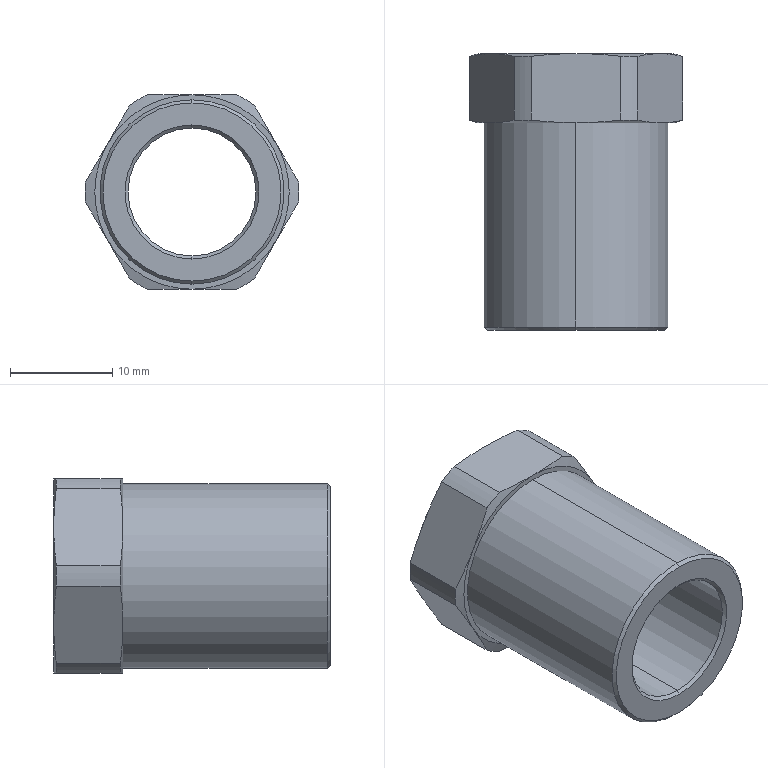Part | STEP file | F_ACA_LM locating stop nut_F-ACA14-LM | 1 solid | 35 faces | box 20.9 x 27 x 19 mm | volume 3920 mm3 | cone 16 | cylinder 10 | plane 9 | commonest cylinder face diameters 20.9 x6 12.5 x2 18 x2